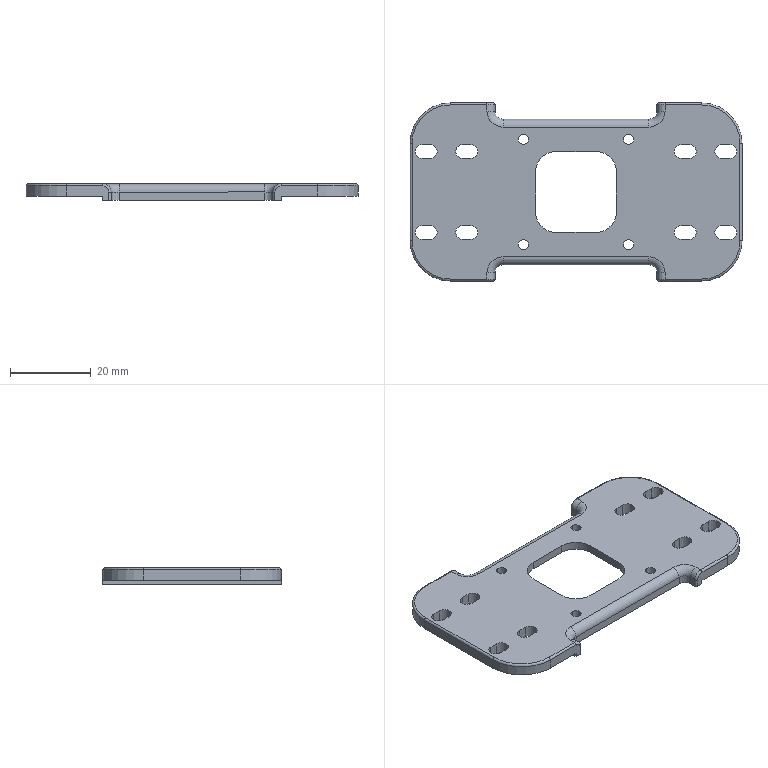NC program | NX | posted with a generic post | part box 82 x 44 x 4 mm
Whole program:
N10 G17 G21 G94 G90
(FLOOR_WALL_COPY , TOOL : D80)
N12 T19 M6
N14 G54
N16 G17 G0 G90 X-84. Y0. S5000 M3
N18 G43 Z30. H19
N20 Z3.
N22 G94 G1 Z0. F1200.
N24 X-81.
N26 X81.
N28 X84.
N30 Z3.
N32 G0 Z30.
N34 M5
(FLOOR_WALL_1 , TOOL : D4)
N36 T11 M6
N38 G54
N40 G17 G0 G90 X-44.5 Y-2.252 S9500 M3
N42 G43 Z30. H11
N44 Z0.7
N46 G94 G1 Z-0.3 F1000.
N48 X-41.2 Y-0.346
N50 G3 X-41. Y0. R0.4
N52 G1 Y12. F2500.
N54 G2 X-31. Y22. R10.
N56 G1 X-24.1
N58 Y-22.
N60 X-31.
N62 G2 X-41. Y-12. R10.
N64 G1 Y0.
N66 X-38.6
N68 Y12.001
N70 G2 X-31. Y19.6 R7.6
N72 G1 X-26.5
N74 Y-19.6
N76 X-31.
N78 G2 X-38.6 Y-12. R7.6
N80 G1 Y0.
N82 X-36.2
N84 Y12.
N86 G2 X-31. Y17.2 R5.2
N88 G1 X-28.9
N90 Y-17.2
N92 X-31.
N94 G2 X-36.2 Y-12. R5.2
N96 G1 Y0.
N98 X-33.8
N100 Y12.
N102 G2 X-31.3 Y14.784 R2.8
N104 G1 Y-14.784
N106 G2 X-33.8 Y-12. R2.8
N108 G1 Y0.
N110 G3 X-34. Y0.347 R0.4
N112 G1 Z0.7
N114 G0 X-44.5 Y-2.252 Z0.4
N116 G1 Z-0.6 F1000.
N118 X-41.2 Y-0.346
N120 G3 X-41. Y0. R0.4
N122 G1 Y12. F2500.
N124 G2 X-31. Y22. R10.
N126 G1 X-24.1
N128 Y-22.
N130 X-31.
N132 G2 X-41. Y-12. R10.
N134 G1 Y0.
N136 X-38.6
N138 Y12.001
N140 G2 X-31. Y19.6 R7.6
N142 G1 X-26.5
N144 Y-19.6
N146 X-31.
N148 G2 X-38.6 Y-12. R7.6
N150 G1 Y0.
N152 X-36.2
N154 Y12.
N156 G2 X-31. Y17.2 R5.2
N158 G1 X-28.9
N160 Y-17.2
N162 X-31.
N164 G2 X-36.2 Y-12. R5.2
N166 G1 Y0.
N168 X-33.8
N170 Y12.
N172 G2 X-31.3 Y14.784 R2.8
N174 G1 Y-14.784
N176 G2 X-33.8 Y-12. R2.8
N178 G1 Y0.
N180 G3 X-34. Y0.347 R0.4
N182 G1 Z0.4
N184 G0 X-44.5 Y-2.252 Z0.1
N186 G1 Z-0.9 F1000.
N188 X-41.2 Y-0.346
N190 G3 X-41. Y0. R0.4
N192 G1 Y12. F2500.
N194 G2 X-31. Y22. R10.
N196 G1 X-24.1
N198 Y-22.
N200 X-31.
N202 G2 X-41. Y-12. R10.
N204 G1 Y0.
N206 X-38.6
N208 Y12.001
N210 G2 X-31. Y19.6 R7.6
N212 G1 X-26.5
N214 Y-19.6
N216 X-31.
N218 G2 X-38.6 Y-12. R7.6
N220 G1 Y0.
N222 X-36.2
N224 Y12.
N226 G2 X-31. Y17.2 R5.2
N228 G1 X-28.9
N230 Y-17.2
N232 X-31.
N234 G2 X-36.2 Y-12. R5.2
N236 G1 Y0.
N238 X-33.8
N240 Y12.
N242 G2 X-31.3 Y14.784 R2.8
N244 G1 Y-14.784
N246 G2 X-33.8 Y-12. R2.8
N248 G1 Y0.
N250 G3 X-34. Y0.347 R0.4
N252 G1 Z0.1
N254 G0 Z30.
N256 X44.5 Y2.252
N258 Z0.7
N260 G1 Z-0.3 F1000.
N262 X41.2 Y0.346
N264 G3 X41. Y0. R0.4
N266 G1 Y-12. F2500.
N268 G2 X31. Y-22. R10.
N270 G1 X24.1
N272 Y22.
N274 X31.
N276 G2 X41. Y12. R10.
N278 G1 Y0.
N280 X38.6
N282 Y-12.
N284 G2 X31. Y-19.6 R7.6
N286 G1 X26.5
N288 Y19.6
N290 X31.
N292 G2 X38.6 Y12. R7.6
N294 G1 Y0.
N296 X36.2
N298 Y-12.
N300 G2 X31. Y-17.2 R5.2
N302 G1 X28.9
N304 Y17.2
N306 X31.
N308 G2 X36.2 Y12. R5.2
N310 G1 Y0.
N312 X33.8
N314 Y-12.
N316 G2 X31.3 Y-14.784 R2.8
N318 G1 Y14.784
N320 G2 X33.8 Y12. R2.8
N322 G1 Y0.
N324 G3 X34. Y-0.346 R0.4
N326 G1 Z0.7
N328 G0 X44.5 Y2.252 Z0.4
N330 G1 Z-0.6 F1000.
N332 X41.2 Y0.346
N334 G3 X41. Y0. R0.4
N336 G1 Y-12. F2500.
N338 G2 X31. Y-22. R10.
N340 G1 X24.1
N342 Y22.
N344 X31.
N346 G2 X41. Y12. R10.
N348 G1 Y0.
N350 X38.6
N352 Y-12.
N354 G2 X31. Y-19.6 R7.6
N356 G1 X26.5
N358 Y19.6
N360 X31.
N362 G2 X38.6 Y12. R7.6
N364 G1 Y0.
N366 X36.2
N368 Y-12.
N370 G2 X31. Y-17.2 R5.2
N372 G1 X28.9
N374 Y17.2
N376 X31.
N378 G2 X36.2 Y12. R5.2
N380 G1 Y0.
N382 X33.8
N384 Y-12.
N386 G2 X31.3 Y-14.784 R2.8
N388 G1 Y14.784
N390 G2 X33.8 Y12. R2.8
N392 G1 Y0.
N394 G3 X34. Y-0.346 R0.4
N396 G1 Z0.4
N398 G0 X44.5 Y2.252 Z0.1
N400 G1 Z-0.9 F1000.
N402 X41.2 Y0.346
N404 G3 X41. Y0. R0.4
N406 G1 Y-12. F2500.
N408 G2 X31. Y-22. R10.
N410 G1 X24.1
N412 Y22.
N414 X31.
N416 G2 X41. Y12. R10.
N418 G1 Y0.
N420 X38.6
N422 Y-12.
N424 G2 X31. Y-19.6 R7.6
N426 G1 X26.5
N428 Y19.6
N430 X31.
N432 G2 X38.6 Y12. R7.6
N434 G1 Y0.
N436 X36.2
N438 Y-12.
N440 G2 X31. Y-17.2 R5.2
N442 G1 X28.9
N444 Y17.2
N446 X31.
N448 G2 X36.2 Y12. R5.2
N450 G1 Y0.
N452 X33.8
N454 Y-12.
N456 G2 X31.3 Y-14.784 R2.8
N458 G1 Y14.784
N460 G2 X33.8 Y12. R2.8
N462 G1 Y0.
N464 G3 X34. Y-0.346 R0.4
N466 G1 Z0.1
N468 G0 Z30.
(FLOOR_WALL_1_COPY , TOOL : D4)
N470 X0.487 Y-0.977
N472 Z0.61
N474 G1 Z-0.39 F700.
N476 G3 X0.873 Y-0.873 R0.4
N478 G2 X1.814 Y0. R17.15 F2500.
N480 X0. Y1.814 R17.15
N482 X-1.814 Y0. R17.15
N484 X0. Y-1.814 R17.15
N486 X0.873 Y-0.873 R17.15
N488 G1 X2.57 Y-2.57
N490 G2 X6.031 Y0. R14.75
N492 X1.053 Y4.35 R14.75
N494 G1 X-1.053
N496 G2 X-6.031 Y0. R14.75
N498 X-1.053 Y-4.35 R14.75
N500 G1 X1.053
N502 G2 X2.57 Y-2.57 R14.75
N504 G1 X4.267 Y-4.267
N506 G2 X10.75 Y-0.857 R12.35
N508 G1 Y0.857
N510 G2 X2.348 Y6.75 R12.35
N512 G1 X-2.348
N514 G2 X-10.75 Y0.857 R12.35
N516 G1 Y-0.857
N518 G2 X-2.348 Y-6.75 R12.35
N520 G1 X2.348
N522 G2 X4.267 Y-4.267 R12.35
N524 G1 X5.964 Y-5.964
N526 G2 X13.15 Y-3.051 R9.95
N528 G1 Y3.051
N530 G2 X3.825 Y9.15 R9.95
N532 G1 X-3.825
N534 G2 X-13.15 Y3.051 R9.95
N536 G1 Y-3.051
N538 G2 X-3.825 Y-9.15 R9.95
N540 G1 X3.825
N542 G2 X5.964 Y-5.964 R9.95
N544 G1 X7.661 Y-7.661
N546 G2 X15.55 Y-5.894 R7.55
N548 G1 Y5.894
N550 G2 X5.591 Y11.55 R7.55
N552 G1 X-5.591
N554 G2 X-15.55 Y5.894 R7.55
N556 G1 Y-5.894
N558 G2 X-5.591 Y-11.55 R7.55
N560 G1 X5.591
N562 G2 X7.661 Y-7.661 R7.55
N564 G1 X9.358 Y-9.358
N566 G2 X17.95 Y-11.579 R5.15
N568 G1 Y11.579
N570 G2 X7.938 Y13.95 R5.15
N572 G1 X-7.938
N574 G2 X-17.95 Y11.579 R5.15
N576 G1 Y-11.579
N578 G2 X-7.938 Y-13.95 R5.15
N580 G1 X7.938
N582 G2 X9.358 Y-9.358 R5.15
N584 G3 X9.462 Y-8.972 R0.4
N586 G1 Z0.61
N588 G0 X0.487 Y-0.977 Z0.22
N590 G1 Z-0.78 F700.
N592 G3 X0.873 Y-0.873 R0.4
N594 G2 X1.814 Y0. R17.15 F2500.
N596 X0. Y1.814 R17.15
N598 X-1.814 Y0. R17.15
N600 X0. Y-1.814 R17.15
N602 X0.873 Y-0.873 R17.15
N604 G1 X2.57 Y-2.57
N606 G2 X6.031 Y0. R14.75
N608 X1.053 Y4.35 R14.75
N610 G1 X-1.053
N612 G2 X-6.031 Y0. R14.75
N614 X-1.053 Y-4.35 R14.75
N616 G1 X1.053
N618 G2 X2.57 Y-2.57 R14.75
N620 G1 X4.267 Y-4.267
N622 G2 X10.75 Y-0.857 R12.35
N624 G1 Y0.857
N626 G2 X2.348 Y6.75 R12.35
N628 G1 X-2.348
N630 G2 X-10.75 Y0.857 R12.35
N632 G1 Y-0.857
N634 G2 X-2.348 Y-6.75 R12.35
N636 G1 X2.348
N638 G2 X4.267 Y-4.267 R12.35
N640 G1 X5.964 Y-5.964
N642 G2 X13.15 Y-3.051 R9.95
N644 G1 Y3.051
N646 G2 X3.825 Y9.15 R9.95
N648 G1 X-3.825
N650 G2 X-13.15 Y3.051 R9.95
N652 G1 Y-3.051
N654 G2 X-3.825 Y-9.15 R9.95
N656 G1 X3.825
N658 G2 X5.964 Y-5.964 R9.95
N660 G1 X7.661 Y-7.661
N662 G2 X15.55 Y-5.894 R7.55
N664 G1 Y5.894
N666 G2 X5.591 Y11.55 R7.55
N668 G1 X-5.591
N670 G2 X-15.55 Y5.894 R7.55
N672 G1 Y-5.894
N674 G2 X-5.591 Y-11.55 R7.55
N676 G1 X5.591
N678 G2 X7.661 Y-7.661 R7.55
N680 G1 X9.358 Y-9.358
N682 G2 X17.95 Y-11.579 R5.15
N684 G1 Y11.579
N686 G2 X7.938 Y13.95 R5.15
N688 G1 X-7.938
N690 G2 X-17.95 Y11.579 R5.15
N692 G1 Y-11.579
N694 G2 X-7.938 Y-13.95 R5.15
N696 G1 X7.938
N698 G2 X9.358 Y-9.358 R5.15
N700 G3 X9.462 Y-8.972 R0.4
N702 G1 Z0.22
N704 G0 X0.487 Y-0.977 Z-0.17
N706 G1 Z-1.17 F700.
N708 G3 X0.873 Y-0.873 R0.4
N710 G2 X1.814 Y0. R17.15 F2500.
N712 X0. Y1.814 R17.15
N714 X-1.814 Y0. R17.15
N716 X0. Y-1.814 R17.15
N718 X0.873 Y-0.873 R17.15
N720 G1 X2.57 Y-2.57
N722 G2 X6.031 Y0. R14.75
N724 X1.053 Y4.35 R14.75
N726 G1 X-1.053
N728 G2 X-6.031 Y0. R14.75
N730 X-1.053 Y-4.35 R14.75
N732 G1 X1.053
N734 G2 X2.57 Y-2.57 R14.75
N736 G1 X4.267 Y-4.267
N738 G2 X10.75 Y-0.857 R12.35
N740 G1 Y0.857
N742 G2 X2.348 Y6.75 R12.35
N744 G1 X-2.348
N746 G2 X-10.75 Y0.857 R12.35
N748 G1 Y-0.857
N750 G2 X-2.348 Y-6.75 R12.35
N752 G1 X2.348
N754 G2 X4.267 Y-4.267 R12.35
N756 G1 X5.964 Y-5.964
N758 G2 X13.15 Y-3.051 R9.95
N760 G1 Y3.051
N762 G2 X3.825 Y9.15 R9.95
N764 G1 X-3.825
N766 G2 X-13.15 Y3.051 R9.95
N768 G1 Y-3.051
N770 G2 X-3.825 Y-9.15 R9.95
N772 G1 X3.825
N774 G2 X5.964 Y-5.964 R9.95
N776 G1 X7.661 Y-7.661
N778 G2 X15.55 Y-5.894 R7.55
N780 G1 Y5.894
N782 G2 X5.591 Y11.55 R7.55
N784 G1 X-5.591
N786 G2 X-15.55 Y5.894 R7.55
N788 G1 Y-5.894
N790 G2 X-5.591 Y-11.55 R7.55
N792 G1 X5.591
N794 G2 X7.661 Y-7.661 R7.55
N796 G1 X9.358 Y-9.358
N798 G2 X17.95 Y-11.579 R5.15
N800 G1 Y11.579
N802 G2 X7.938 Y13.95 R5.15
N804 G1 X-7.938
N806 G2 X-17.95 Y11.579 R5.15
N808 G1 Y-11.579
N810 G2 X-7.938 Y-13.95 R5.15
N812 G1 X7.938
N814 G2 X9.358 Y-9.358 R5.15
N816 G3 X9.462 Y-8.972 R0.4
N818 G1 Z-0.17
N820 G0 X0.487 Y-0.977 Z-0.56
N822 G1 Z-1.56 F700.
N824 G3 X0.873 Y-0.873 R0.4
N826 G2 X1.814 Y0. R17.15 F2500.
N828 X0. Y1.814 R17.15
N830 X-1.814 Y0. R17.15
N832 X0. Y-1.814 R17.15
N834 X0.873 Y-0.873 R17.15
N836 G1 X2.57 Y-2.57
N838 G2 X6.031 Y0. R14.75
N840 X1.053 Y4.35 R14.75
N842 G1 X-1.053
N844 G2 X-6.031 Y0. R14.75
N846 X-1.053 Y-4.35 R14.75
N848 G1 X1.053
N850 G2 X2.57 Y-2.57 R14.75
N852 G1 X4.267 Y-4.267
N854 G2 X10.75 Y-0.857 R12.35
N856 G1 Y0.857
N858 G2 X2.348 Y6.75 R12.35
N860 G1 X-2.348
N862 G2 X-10.75 Y0.857 R12.35
N864 G1 Y-0.857
N866 G2 X-2.348 Y-6.75 R12.35
N868 G1 X2.348
N870 G2 X4.267 Y-4.267 R12.35
N872 G1 X5.964 Y-5.964
N874 G2 X13.15 Y-3.051 R9.95
N876 G1 Y3.051
N878 G2 X3.825 Y9.15 R9.95
N880 G1 X-3.825
N882 G2 X-13.15 Y3.051 R9.95
N884 G1 Y-3.051
N886 G2 X-3.825 Y-9.15 R9.95
N888 G1 X3.825
N890 G2 X5.964 Y-5.964 R9.95
N892 G1 X7.661 Y-7.661
N894 G2 X15.55 Y-5.894 R7.55
N896 G1 Y5.894
N898 G2 X5.591 Y11.55 R7.55
N900 G1 X-5.591
N902 G2 X-15.55 Y5.894 R7.55
N904 G1 Y-5.894
N906 G2 X-5.591 Y-11.55 R7.55
N908 G1 X5.591
N910 G2 X7.661 Y-7.661 R7.55
N912 G1 X9.358 Y-9.358
N914 G2 X17.95 Y-11.579 R5.15
N916 G1 Y11.579
N918 G2 X7.938 Y13.95 R5.15
N920 G1 X-7.938
N922 G2 X-17.95 Y11.579 R5.15
N924 G1 Y-11.579
N926 G2 X-7.938 Y-13.95 R5.15
N928 G1 X7.938
N930 G2 X9.358 Y-9.358 R5.15
N932 G3 X9.462 Y-8.972 R0.4
N934 G1 Z-0.56
N936 G0 X0.487 Y-0.977 Z-0.95
N938 G1 Z-1.95 F700.
N940 G3 X0.873 Y-0.873 R0.4
N942 G2 X1.814 Y0. R17.15 F2500.
N944 X0. Y1.814 R17.15
N946 X-1.814 Y0. R17.15
N948 X0. Y-1.814 R17.15
N950 X0.873 Y-0.873 R17.15
N952 G1 X2.57 Y-2.57
N954 G2 X6.031 Y0. R14.75
N956 X1.053 Y4.35 R14.75
N958 G1 X-1.053
N960 G2 X-6.031 Y0. R14.75
N962 X-1.053 Y-4.35 R14.75
N964 G1 X1.053
N966 G2 X2.57 Y-2.57 R14.75
N968 G1 X4.267 Y-4.267
N970 G2 X10.75 Y-0.857 R12.35
N972 G1 Y0.857
N974 G2 X2.348 Y6.75 R12.35
N976 G1 X-2.348
N978 G2 X-10.75 Y0.857 R12.35
N980 G1 Y-0.857
N982 G2 X-2.348 Y-6.75 R12.35
N984 G1 X2.348
N986 G2 X4.267 Y-4.267 R12.35
N988 G1 X5.964 Y-5.964
N990 G2 X13.15 Y-3.051 R9.95
N992 G1 Y3.051
N994 G2 X3.825 Y9.15 R9.95
N996 G1 X-3.825
N998 G2 X-13.15 Y3.051 R9.95
N1000 G1 Y-3.051
N1002 G2 X-3.825 Y-9.15 R9.95
N1004 G1 X3.825
N1006 G2 X5.964 Y-5.964 R9.95
N1008 G1 X7.661 Y-7.661
N1010 G2 X15.55 Y-5.894 R7.55
N1012 G1 Y5.894
N1014 G2 X5.591 Y11.55 R7.55
N1016 G1 X-5.591
N1018 G2 X-15.55 Y5.894 R7.55
N1020 G1 Y-5.894
N1022 G2 X-5.591 Y-11.55 R7.55
N1024 G1 X5.591
N1026 G2 X7.661 Y-7.661 R7.55
N1028 G1 X9.358 Y-9.358
N1030 G2 X17.95 Y-11.579 R5.15
N1032 G1 Y11.579
N1034 G2 X7.938 Y13.95 R5.15
N1036 G1 X-7.938
N1038 G2 X-17.95 Y11.579 R5.15
N1040 G1 Y-11.579
N1042 G2 X-7.938 Y-13.95 R5.15
N1044 G1 X7.938
N1046 G2 X9.358 Y-9.358 R5.15
N1048 G3 X9.462 Y-8.972 R0.4
N1050 G1 Z-0.95
N1052 G0 Z30.
(FLOOR_WALL_1_COPY_COPY , TOOL : D4)
N1054 X44.5 Y1.097
N1056 Z0.
N1058 G1 Z-1. F700.
N1060 X43.2 Y0.346
N1062 G3 X43. Y0. R0.4
N1064 G1 Y-12. F1300.
N1066 G2 X31. Y-24. R12.
N1068 G1 X24.2
N1070 Y24.
N1072 X31.
N1074 G2 X43. Y12. R12.
N1076 G1 Y0.
N1078 X40.6
N1080 Y-12.
N1082 G2 X31. Y-21.6 R9.6
N1084 G1 X26.6
N1086 Y21.6
N1088 X31.
N1090 G2 X40.6 Y12. R9.6
N1092 G1 Y0.
N1094 X38.2
N1096 Y-12.
N1098 G2 X31. Y-19.2 R7.2
N1100 G1 X29.
N1102 Y19.2
N1104 X31.
N1106 G2 X38.2 Y12. R7.2
N1108 G1 Y0.
N1110 X35.8
N1112 Y-12.
N1114 G2 X31.4 Y-16.783 R4.8
N1116 G1 Y16.783
N1118 G2 X35.8 Y12. R4.8
N1120 G1 Y0.
N1122 X34.
N1124 Y-12.
N1126 G2 X33.2 Y-14.04 R3.
N1128 G1 Y14.04
N1130 G2 X34. Y12. R3.
N1132 G1 Y0.
N1134 G3 X34.2 Y-0.346 R0.4
N1136 G1 Z0.
N1138 G0 X26.198 Y25.5
N1140 G1 Z-1. F700.
N1142 X24.2 Y24.346
N1144 G3 X24. Y24. R0.4
N1146 G1 Y-24. F1300.
N1148 G3 X24.2 Y-24.346 R0.4
N1150 G1 X26.198 Y-25.5
N1152 Z0.
N1154 G0 Z30.
N1156 X9.356 Y8.866
N1158 Z-1.
N1160 G1 Z-2. F700.
N1162 G3 X9.252 Y9.252 R0.4
N1164 X17.8 Y10.753 R5.3 F1300.
N1166 G1 Y-10.753
N1168 G3 X7.761 Y-13.8 R5.3
N1170 G1 X-7.761
N1172 G3 X-17.8 Y-10.753 R5.3
N1174 G1 Y10.753
N1176 G3 X-7.761 Y13.8 R5.3
N1178 G1 X7.761
N1180 G3 X9.252 Y9.252 R5.3
N1182 G1 X7.555 Y7.555
N1184 G3 X15.4 Y5.684 R7.7
N1186 G1 Y-5.684
N1188 G3 X5.468 Y-11.4 R7.7
N1190 G1 X-5.468
N1192 G3 X-15.4 Y-5.684 R7.7
N1194 G1 Y5.684
N1196 G3 X-5.468 Y11.4 R7.7
N1198 G1 X5.468
N1200 G3 X7.555 Y7.555 R7.7
N1202 G1 X5.858 Y5.858
N1204 G3 X13. Y2.9 R10.1
N1206 G1 Y-2.9
N1208 G3 X3.726 Y-9. R10.1
N1210 G1 X-3.726
N1212 G3 X-13. Y-2.9 R10.1
N1214 G1 Y2.9
N1216 G3 X-3.726 Y9. R10.1
N1218 G1 X3.726
N1220 G3 X5.858 Y5.858 R10.1
N1222 G1 X4.161 Y4.161
N1224 G3 X10.6 Y0.733 R12.5
N1226 G1 Y-0.733
N1228 G3 X2.263 Y-6.6 R12.5
N1230 G1 X-2.263
N1232 G3 X-10.6 Y-0.733 R12.5
N1234 G1 Y0.733
N1236 G3 X-2.263 Y6.6 R12.5
N1238 G1 X2.263
N1240 G3 X4.161 Y4.161 R12.5
N1242 G1 X2.464 Y2.464
N1244 G3 X5.719 Y0. R14.9
N1246 X0.976 Y-4.2 R14.9
N1248 G1 X-0.976
N1250 G3 X-5.719 Y0. R14.9
N1252 X-0.976 Y4.2 R14.9
N1254 G1 X0.976
N1256 G3 X2.464 Y2.464 R14.9
N1258 G1 X0.767 Y0.767
N1260 G3 X1.586 Y0. R17.3
N1262 X0. Y-1.586 R17.3
N1264 X-1.586 Y0. R17.3
N1266 X0. Y1.586 R17.3
N1268 X0.767 Y0.767 R17.3
N1270 X1.153 Y0.664 R0.4
N1272 G1 Z-1.
N1274 G0 X16.3 Y-1.212
N1276 G1 Z-2. F700.
N1278 X17.8 Y-0.346
N1280 G3 X18. Y0. R0.4
N1282 G1 Y11.995 F1300.
N1284 G2 X11.995 Y8. R5.1
N1286 X7.999 Y14. R5.1
N1288 G1 X-7.999
N1290 G2 X-12. Y7.999 R5.1
N1292 X-18. Y11.995 R5.1
N1294 G1 Y-11.995
N1296 G2 X-11.995 Y-8. R5.1
N1298 X-7.999 Y-14. R5.1
N1300 G1 X7.999
N1302 G2 X12. Y-7.999 R5.1
N1304 X18. Y-11.995 R5.1
N1306 G1 Y0.
N1308 G3 X17.8 Y0.346 R0.4
N1310 G1 X16.5 Y1.097
N1312 Z-1.
N1314 G0 Z30.
N1316 X-44.5 Y-1.097
N1318 Z0.
N1320 G1 Z-1. F700.
N1322 X-43.2 Y-0.346
N1324 G3 X-43. Y0. R0.4
N1326 G1 Y12. F1300.
N1328 G2 X-31. Y24. R12.
N1330 G1 X-24.2
N1332 Y-24.
N1334 X-31.
N1336 G2 X-43. Y-12. R12.
N1338 G1 Y0.
N1340 X-40.6
N1342 Y12.
N1344 G2 X-31. Y21.6 R9.6
N1346 G1 X-26.6
N1348 Y-21.6
N1350 X-31.
N1352 G2 X-40.6 Y-12. R9.6
N1354 G1 Y0.
N1356 X-38.2
N1358 Y12.001
N1360 G2 X-31. Y19.2 R7.2
N1362 G1 X-29.
N1364 Y-19.2
N1366 X-31.
N1368 G2 X-38.2 Y-12. R7.2
N1370 G1 Y0.
N1372 X-35.8
N1374 Y12.001
N1376 G2 X-31.4 Y16.783 R4.8
N1378 G1 Y-16.783
N1380 G2 X-35.8 Y-12. R4.8
N1382 G1 Y0.
N1384 X-34.
N1386 Y12.
N1388 G2 X-33.2 Y14.04 R3.
N1390 G1 Y-14.04
N1392 G2 X-34. Y-12. R3.
N1394 G1 Y0.
N1396 G3 X-34.2 Y0.347 R0.4
N1398 G1 Z0.
N1400 G0 X-26.198 Y-25.5
N1402 G1 Z-1. F700.
N1404 X-24.2 Y-24.346
N1406 G3 X-24. Y-24. R0.4
N1408 G1 Y24. F1300.
N1410 G3 X-24.2 Y24.346 R0.4
N1412 G1 X-26.198 Y25.5
N1414 Z0.
N1416 G0 Z30.
N1418 M5
(ZLEVEL_PROFILE_COPY_1_COPY , TOOL : D3)
N1420 T16 M6
N1422 G54
N1424 G17 G0 G90 X-17.9 Y-11.092 S9500 M3
N1426 G43 Z30. H16
N1428 Z1.214
N1430 G94 G1 Z-0.286 F1000.
N1432 X-18.35 Y-11.352
N1434 G3 X-18.5 Y-11.612 R0.3
N1436 G1 Y-14. F1200.
N1438 G3 X-18. Y-14.5 R0.5
N1440 X-17.511 Y-13.902 R0.5
N1442 G2 X-17.412 Y-11.699 R4.6
N1444 G3 X-17.483 Y-11.408 R0.3
N1446 G1 X-17.821 Y-11.052
N1448 Z1.214
N1450 G0 X-17.9 Y-11.092 Z0.929
N1452 G1 Z-0.571 F1000.
N1454 X-18.35 Y-11.352
N1456 G3 X-18.5 Y-11.612 R0.3
N1458 G1 Y-14. F1200.
N1460 G3 X-18. Y-14.5 R0.5
N1462 X-17.511 Y-13.902 R0.5
N1464 G2 X-17.412 Y-11.699 R4.6
N1466 G3 X-17.483 Y-11.408 R0.3
N1468 G1 X-17.821 Y-11.052
N1470 Z0.929
N1472 G0 X-17.9 Y-11.092 Z0.643
N1474 G1 Z-0.857 F1000.
N1476 X-18.35 Y-11.352
N1478 G3 X-18.5 Y-11.612 R0.3
N1480 G1 Y-14. F1200.
N1482 G3 X-18. Y-14.5 R0.5
N1484 X-17.511 Y-13.902 R0.5
N1486 G2 X-17.412 Y-11.699 R4.6
N1488 G3 X-17.483 Y-11.408 R0.3
N1490 G1 X-17.821 Y-11.052
N1492 Z0.643
N1494 G0 X-17.9 Y-11.092 Z0.357
N1496 G1 Z-1.143 F1000.
N1498 X-18.35 Y-11.352
N1500 G3 X-18.5 Y-11.612 R0.3
N1502 G1 Y-14. F1200.
N1504 G3 X-18. Y-14.5 R0.5
N1506 X-17.511 Y-13.902 R0.5
N1508 G2 X-17.412 Y-11.699 R4.6
N1510 G3 X-17.483 Y-11.408 R0.3
N1512 G1 X-17.821 Y-11.052
N1514 Z0.357
N1516 G0 X-17.9 Y-11.092 Z0.071
N1518 G1 Z-1.429 F1000.
N1520 X-18.35 Y-11.352
N1522 G3 X-18.5 Y-11.612 R0.3
N1524 G1 Y-14. F1200.
N1526 G3 X-18. Y-14.5 R0.5
N1528 X-17.511 Y-13.902 R0.5
N1530 G2 X-17.412 Y-11.699 R4.6
N1532 G3 X-17.483 Y-11.408 R0.3
N1534 G1 X-17.821 Y-11.052
N1536 Z0.071
N1538 G0 X-17.9 Y-11.092 Z-0.214
N1540 G1 Z-1.714 F1000.
N1542 X-18.35 Y-11.352
N1544 G3 X-18.5 Y-11.612 R0.3
N1546 G1 Y-14. F1200.
N1548 G3 X-18. Y-14.5 R0.5
N1550 X-17.511 Y-13.902 R0.5
N1552 G2 X-17.412 Y-11.699 R4.6
N1554 G3 X-17.483 Y-11.408 R0.3
N1556 G1 X-17.821 Y-11.052
N1558 Z-0.214
N1560 G0 X-17.9 Y-11.092 Z-0.5
N1562 G1 Z-2. F1000.
N1564 X-18.35 Y-11.352
N1566 G3 X-18.5 Y-11.612 R0.3
N1568 G1 Y-14. F1200.
N1570 G3 X-18. Y-14.5 R0.5
N1572 X-17.511 Y-13.902 R0.5
N1574 G2 X-17.412 Y-11.699 R4.6
N1576 G3 X-17.483 Y-11.408 R0.3
N1578 G1 X-17.821 Y-11.052
N1580 Z-0.5
N1582 G0 Z30.
N1584 X17.839 Y-11.096
N1586 Z1.214
N1588 G1 Z-0.286 F1000.
N1590 X17.497 Y-11.448
N1592 G3 X17.424 Y-11.739 R0.3
N1594 G2 X17.511 Y-13.902 R4.6 F1200.
N1596 G3 X18. Y-14.5 R0.5
N1598 X18.5 Y-14. R0.5
N1600 G1 Y-11.638
N1602 G3 X18.35 Y-11.378 R0.3
N1604 G1 X17.9 Y-11.118
N1606 Z1.214
N1608 G0 X17.839 Y-11.096 Z0.929
N1610 G1 Z-0.571 F1000.
N1612 X17.497 Y-11.448
N1614 G3 X17.424 Y-11.739 R0.3
N1616 G2 X17.511 Y-13.902 R4.6 F1200.
N1618 G3 X18. Y-14.5 R0.5
N1620 X18.5 Y-14. R0.5
N1622 G1 Y-11.638
N1624 G3 X18.35 Y-11.378 R0.3
N1626 G1 X17.9 Y-11.118
N1628 Z0.929
N1630 G0 X17.839 Y-11.096 Z0.643
N1632 G1 Z-0.857 F1000.
N1634 X17.497 Y-11.448
N1636 G3 X17.424 Y-11.739 R0.3
N1638 G2 X17.511 Y-13.902 R4.6 F1200.
N1640 G3 X18. Y-14.5 R0.5
N1642 X18.5 Y-14. R0.5
N1644 G1 Y-11.638
N1646 G3 X18.35 Y-11.378 R0.3
N1648 G1 X17.9 Y-11.118
N1650 Z0.643
N1652 G0 X17.839 Y-11.096 Z0.357
N1654 G1 Z-1.143 F1000.
N1656 X17.497 Y-11.448
N1658 G3 X17.424 Y-11.739 R0.3
N1660 G2 X17.511 Y-13.902 R4.6 F1200.
N1662 G3 X18. Y-14.5 R0.5
N1664 X18.5 Y-14. R0.5
N1666 G1 Y-11.638
N1668 G3 X18.35 Y-11.378 R0.3
N1670 G1 X17.9 Y-11.118
N1672 Z0.357
N1674 G0 X17.839 Y-11.096 Z0.071
N1676 G1 Z-1.429 F1000.
N1678 X17.497 Y-11.448
N1680 G3 X17.424 Y-11.739 R0.3
N1682 G2 X17.511 Y-13.902 R4.6 F1200.
N1684 G3 X18. Y-14.5 R0.5
N1686 X18.5 Y-14. R0.5
N1688 G1 Y-11.638
N1690 G3 X18.35 Y-11.378 R0.3
N1692 G1 X17.9 Y-11.118
N1694 Z0.071
N1696 G0 X17.839 Y-11.096 Z-0.214
N1698 G1 Z-1.714 F1000.
N1700 X17.497 Y-11.448
N1702 G3 X17.424 Y-11.739 R0.3
N1704 G2 X17.511 Y-13.902 R4.6 F1200.
N1706 G3 X18. Y-14.5 R0.5
N1708 X18.5 Y-14. R0.5
N1710 G1 Y-11.638
N1712 G3 X18.35 Y-11.378 R0.3
N1714 G1 X17.9 Y-11.118
N1716 Z-0.214
N1718 G0 X17.839 Y-11.096 Z-0.5
N1720 G1 Z-2. F1000.
N1722 X17.497 Y-11.448
N1724 G3 X17.424 Y-11.739 R0.3
N1726 G2 X17.511 Y-13.902 R4.6 F1200.
N1728 G3 X18. Y-14.5 R0.5
N1730 X18.5 Y-14. R0.5
N1732 G1 Y-11.638
N1734 G3 X18.35 Y-11.378 R0.3
N1736 G1 X17.9 Y-11.118
N1738 Z-0.5
N1740 G0 Z30.
N1742 Y11.092
N1744 Z1.214
N1746 G1 Z-0.286 F1000.
N1748 X18.35 Y11.352
N1750 G3 X18.5 Y11.612 R0.3
N1752 G1 Y14. F1200.
N1754 G3 X18. Y14.5 R0.5
N1756 X17.511 Y13.902 R0.5
N1758 G2 X17.412 Y11.699 R4.6
N1760 G3 X17.483 Y11.408 R0.3
N1762 G1 X17.821 Y11.052
N1764 Z1.214
N1766 G0 X17.9 Y11.092 Z0.929
N1768 G1 Z-0.571 F1000.
N1770 X18.35 Y11.352
N1772 G3 X18.5 Y11.612 R0.3
N1774 G1 Y14. F1200.
N1776 G3 X18. Y14.5 R0.5
N1778 X17.511 Y13.902 R0.5
N1780 G2 X17.412 Y11.699 R4.6
N1782 G3 X17.483 Y11.408 R0.3
N1784 G1 X17.821 Y11.052
N1786 Z0.929
N1788 G0 X17.9 Y11.092 Z0.643
N1790 G1 Z-0.857 F1000.
N1792 X18.35 Y11.352
N1794 G3 X18.5 Y11.612 R0.3
N1796 G1 Y14. F1200.
N1798 G3 X18. Y14.5 R0.5
N1800 X17.511 Y13.902 R0.5
N1802 G2 X17.412 Y11.699 R4.6
N1804 G3 X17.483 Y11.408 R0.3
N1806 G1 X17.821 Y11.052
N1808 Z0.643
N1810 G0 X17.9 Y11.092 Z0.357
N1812 G1 Z-1.143 F1000.
N1814 X18.35 Y11.352
N1816 G3 X18.5 Y11.612 R0.3
N1818 G1 Y14. F1200.
N1820 G3 X18. Y14.5 R0.5
N1822 X17.511 Y13.902 R0.5
N1824 G2 X17.412 Y11.699 R4.6
N1826 G3 X17.483 Y11.408 R0.3
N1828 G1 X17.821 Y11.052
N1830 Z0.357
N1832 G0 X17.9 Y11.092 Z0.071
N1834 G1 Z-1.429 F1000.
N1836 X18.35 Y11.352
N1838 G3 X18.5 Y11.612 R0.3
N1840 G1 Y14. F1200.
N1842 G3 X18. Y14.5 R0.5
N1844 X17.511 Y13.902 R0.5
N1846 G2 X17.412 Y11.699 R4.6
N1848 G3 X17.483 Y11.408 R0.3
N1850 G1 X17.821 Y11.052
N1852 Z0.071
N1854 G0 X17.9 Y11.092 Z-0.214
N1856 G1 Z-1.714 F1000.
N1858 X18.35 Y11.352
N1860 G3 X18.5 Y11.612 R0.3
N1862 G1 Y14. F1200.
N1864 G3 X18. Y14.5 R0.5
N1866 X17.511 Y13.902 R0.5
N1868 G2 X17.412 Y11.699 R4.6
N1870 G3 X17.483 Y11.408 R0.3
N1872 G1 X17.821 Y11.052
N1874 Z-0.214
N1876 G0 X17.9 Y11.092 Z-0.5
N1878 G1 Z-2. F1000.
N1880 X18.35 Y11.352
N1882 G3 X18.5 Y11.612 R0.3
N1884 G1 Y14. F1200.
N1886 G3 X18. Y14.5 R0.5
N1888 X17.511 Y13.902 R0.5
N1890 G2 X17.412 Y11.699 R4.6
N1892 G3 X17.483 Y11.408 R0.3
N1894 G1 X17.821 Y11.052
N1896 Z-0.5
N1898 G0 Z30.
N1900 X-17.839 Y11.096
N1902 Z1.214
N1904 G1 Z-0.286 F1000.
N1906 X-17.497 Y11.448
N1908 G3 X-17.424 Y11.739 R0.3
N1910 G2 X-17.511 Y13.902 R4.6 F1200.
N1912 G3 X-18. Y14.5 R0.5
N1914 X-18.5 Y14. R0.5
N1916 G1 Y11.638
N1918 G3 X-18.35 Y11.378 R0.3
N1920 G1 X-17.9 Y11.118
N1922 Z1.214
N1924 G0 X-17.839 Y11.096 Z0.929
N1926 G1 Z-0.571 F1000.
N1928 X-17.497 Y11.448
N1930 G3 X-17.424 Y11.739 R0.3
N1932 G2 X-17.511 Y13.902 R4.6 F1200.
N1934 G3 X-18. Y14.5 R0.5
N1936 X-18.5 Y14. R0.5
N1938 G1 Y11.638
N1940 G3 X-18.35 Y11.378 R0.3
N1942 G1 X-17.9 Y11.118
N1944 Z0.929
N1946 G0 X-17.839 Y11.096 Z0.643
N1948 G1 Z-0.857 F1000.
N1950 X-17.497 Y11.448
N1952 G3 X-17.424 Y11.739 R0.3
N1954 G2 X-17.511 Y13.902 R4.6 F1200.
N1956 G3 X-18. Y14.5 R0.5
N1958 X-18.5 Y14. R0.5
N1960 G1 Y11.638
N1962 G3 X-18.35 Y11.378 R0.3
N1964 G1 X-17.9 Y11.118
N1966 Z0.643
N1968 G0 X-17.839 Y11.096 Z0.357
N1970 G1 Z-1.143 F1000.
N1972 X-17.497 Y11.448
N1974 G3 X-17.424 Y11.739 R0.3
N1976 G2 X-17.511 Y13.902 R4.6 F1200.
N1978 G3 X-18. Y14.5 R0.5
N1980 X-18.5 Y14. R0.5
N1982 G1 Y11.638
N1984 G3 X-18.35 Y11.378 R0.3
N1986 G1 X-17.9 Y11.118
N1988 Z0.357
N1990 G0 X-17.839 Y11.096 Z0.071
N1992 G1 Z-1.429 F1000.
N1994 X-17.497 Y11.448
N1996 G3 X-17.424 Y11.739 R0.3
N1998 G2 X-17.511 Y13.902 R4.6 F1200.
N2000 G3 X-18. Y14.5 R0.5
N2002 X-18.5 Y14. R0.5
N2004 G1 Y11.638
N2006 G3 X-18.35 Y11.378 R0.3
N2008 G1 X-17.9 Y11.118
N2010 Z0.071
N2012 G0 X-17.839 Y11.096 Z-0.214
N2014 G1 Z-1.714 F1000.
N2016 X-17.497 Y11.448
N2018 G3 X-17.424 Y11.739 R0.3
N2020 G2 X-17.511 Y13.902 R4.6 F1200.
N2022 G3 X-18. Y14.5 R0.5
N2024 X-18.5 Y14. R0.5
N2026 G1 Y11.638
N2028 G3 X-18.35 Y11.378 R0.3
N2030 G1 X-17.9 Y11.118
N2032 Z-0.214
N2034 G0 X-17.839 Y11.096 Z-0.5
N2036 G1 Z-2. F1000.
N2038 X-17.497 Y11.448
N2040 G3 X-17.424 Y11.739 R0.3
N2042 G2 X-17.511 Y13.902 R4.6 F1200.
N2044 G3 X-18. Y14.5 R0.5
N2046 X-18.5 Y14. R0.5
N2048 G1 Y11.638
N2050 G3 X-18.35 Y11.378 R0.3
N2052 G1 X-17.9 Y11.118
N2054 Z-0.5
N2056 G0 Z30.
N2058 M5
(PLANAR_MILL_2_COPY_COPY , TOOL : D6A45)
N2060 T01 M6
N2062 G54
N2064 G17 G0 G90 X-13.6 Y13.433 S9500 M3
N2066 G43 Z30. H1
N2068 Z0.5
N2070 G94 G1 Z-0.5 F1250.
N2072 G3 X-13.85 Y13. R0.5
N2074 X-13. Y12.15 R0.85
N2076 X-13.85 Y13. R-0.85
N2078 X-13.6 Y12.567 R0.5
N2080 G1 Z0.5
N2082 G0 Z30.
N2084 X-19.1 Y0.866
N2086 Z0.5
N2088 G1 Z-0.5
N2090 G3 X-19.6 Y0. R1.
N2092 G1 Y-14.
N2094 G3 X-18. Y-15.6 R1.6
N2096 X-16.432 Y-13.686 R1.6
N2098 G2 X-9.568 Y-13.686 R-3.5
N2100 G3 X-7.999 Y-15.6 R1.6
N2102 G1 X7.999
N2104 G3 X9.568 Y-13.686 R1.6
N2106 G2 X16.432 Y-13.686 R-3.5
N2108 G3 X18. Y-15.6 R1.6
N2110 X19.6 Y-14. R1.6
N2112 G1 Y14.
N2114 G3 X18. Y15.6 R1.6
N2116 X16.432 Y13.686 R1.6
N2118 G2 X9.568 Y13.686 R-3.5
N2120 G3 X7.999 Y15.6 R1.6
N2122 G1 X-7.999
N2124 G3 X-9.568 Y13.686 R1.6
N2126 G2 X-16.432 Y13.686 R-3.5
N2128 G3 X-18. Y15.6 R1.6
N2130 X-19.6 Y14. R1.6
N2132 G1 Y0.
N2134 G3 X-19.1 Y-0.866 R1.
N2136 G1 Z0.5
N2138 G0 Z30.
N2140 X13.6 Y12.567
N2142 Z0.5
N2144 G1 Z-0.5
N2146 G3 X13.85 Y13. R0.5
N2148 X13. Y13.85 R0.85
N2150 X13.85 Y13. R-0.85
N2152 X13.6 Y13.433 R0.5
N2154 G1 Z0.5
N2156 G0 Z30.
N2158 X22.9 Y0.866
N2160 Z0.5
N2162 G1 Z-0.5
N2164 G3 X22.4 Y0. R1.
N2166 G1 Y-22.
N2168 G2 X22. Y-22.4 R0.4
N2170 G1 X20.5
N2172 G2 X19.6 Y-21.5 R0.9
N2174 G1 Y-20.
N2176 G3 X18. Y-18.4 R1.6
N2178 G1 X-18.
N2180 G3 X-19.6 Y-20. R1.6
N2182 G1 Y-21.5
N2184 G2 X-20.5 Y-22.4 R0.9
N2186 G1 X-22.
N2188 G2 X-22.4 Y-22. R0.4
N2190 G1 Y22.
N2192 G2 X-22. Y22.4 R0.4
N2194 G1 X-20.5
N2196 G2 X-19.6 Y21.5 R0.9
N2198 G1 Y20.
N2200 G3 X-18. Y18.4 R1.6
N2202 G1 X18.
N2204 G3 X19.6 Y20. R1.6
N2206 G1 Y21.5
N2208 G2 X20.5 Y22.4 R0.9
N2210 G1 X22.
N2212 G2 X22.4 Y22. R0.4
N2214 G1 Y0.
N2216 G3 X22.9 Y-0.866 R1.
N2218 G1 Z0.5
N2220 G0 Z30.
N2222 X13.6 Y-13.433
N2224 Z0.5
N2226 G1 Z-0.5
N2228 G3 X13.85 Y-13. R0.5
N2230 X13. Y-12.15 R0.85
N2232 X13.85 Y-13. R-0.85
N2234 X13.6 Y-12.567 R0.5
N2236 G1 Z0.5
N2238 G0 Z30.
N2240 X-13.6
N2242 Z0.5
N2244 G1 Z-0.5
N2246 G3 X-13.85 Y-13. R0.5
N2248 X-13. Y-13.85 R0.85
N2250 X-13.85 Y-13. R-0.85
N2252 X-13.6 Y-13.433 R0.5
N2254 G1 Z0.5
N2256 G0 Z30.
(PLANAR_MILL_2_COPY_COPY_COPY , TOOL : D6A45)
N2258 X-9.1 Y0.866
N2260 Z-1.5
N2262 G1 Z-2.5
N2264 G3 X-9.6 Y0. R1.
N2266 G1 Y-5.
N2268 G3 X-5. Y-9.6 R4.6
N2270 G1 X5.
N2272 G3 X9.6 Y-5. R4.6
N2274 G1 Y5.
N2276 G3 X5. Y9.6 R4.6
N2278 G1 X-5.
N2280 G3 X-9.6 Y5. R4.6
N2282 G1 Y0.
N2284 G3 X-9.1 Y-0.866 R1.
N2286 G1 Z-1.5
N2288 G0 Z30.
(PLANAR_MILL_2_COPY_COPY_COPY_COPY , TOOL : D6A45)
N2290 X-26.699 Y10.3
N2292 Z0.
N2294 G1 X-28.137 Z-0.386
N2296 X-28.3 Y10.137 Z-0.447
N2298 Y9.863 Z-0.521
N2300 X-28.137 Y9.7 Z-0.582
N2302 X-25.863 Z-1.192
N2304 X-25.7 Y9.863 Z-1.254
N2306 Y10.137 Z-1.327
N2308 X-25.863 Y10.3 Z-1.389
N2310 X-28.137 Z-1.998
N2312 X-28.3 Y10.137 Z-2.06
N2314 Y9.863 Z-2.134
N2316 X-28.137 Y9.7 Z-2.195
N2318 X-27. Z-2.5
N2320 X-26.
N2322 G3 X-25.7 Y10. R0.3
N2324 X-26. Y10.3 R0.3
N2326 G1 X-28.
N2328 G3 X-28.3 Y10. R0.3
N2330 X-28. Y9.7 R0.3
N2332 G1 X-27.
N2334 G3 X-26.134 Y10.2 R1.
N2336 G1 Z-1.5
N2338 G0 Z30.
N2340 X-36.699 Y10.3
N2342 Z0.
N2344 G1 X-38.137 Z-0.386
N2346 X-38.3 Y10.137 Z-0.447
N2348 Y9.863 Z-0.521
N2350 X-38.137 Y9.7 Z-0.582
N2352 X-35.863 Z-1.192
N2354 X-35.7 Y9.863 Z-1.254
N2356 Y10.137 Z-1.327
N2358 X-35.863 Y10.3 Z-1.389
N2360 X-38.137 Z-1.998
N2362 X-38.3 Y10.137 Z-2.06
N2364 Y9.863 Z-2.134
N2366 X-38.137 Y9.7 Z-2.195
N2368 X-37. Z-2.5
N2370 X-36.
N2372 G3 X-35.7 Y10. R0.3
N2374 X-36. Y10.3 R0.3
N2376 G1 X-38.
N2378 G3 X-38.3 Y10. R0.3
N2380 X-38. Y9.7 R0.3
N2382 G1 X-37.
N2384 G3 X-36.134 Y10.2 R1.
N2386 G1 Z-1.5
N2388 G0 Z30.
N2390 X-37.301 Y-10.3
N2392 Z0.
N2394 G1 X-35.863 Z-0.386
N2396 X-35.7 Y-10.137 Z-0.447
N2398 Y-9.863 Z-0.521
N2400 X-35.863 Y-9.7 Z-0.582
N2402 X-38.137 Z-1.192
N2404 X-38.3 Y-9.863 Z-1.254
N2406 Y-10.137 Z-1.327
N2408 X-38.137 Y-10.3 Z-1.389
N2410 X-35.863 Z-1.998
N2412 X-35.7 Y-10.137 Z-2.06
N2414 Y-9.863 Z-2.134
N2416 X-35.863 Y-9.7 Z-2.195
N2418 X-37. Z-2.5
N2420 X-38.
N2422 G3 X-38.3 Y-10. R0.3
N2424 X-38. Y-10.3 R0.3
N2426 G1 X-36.
N2428 G3 X-35.7 Y-10. R0.3
N2430 X-36. Y-9.7 R0.3
N2432 G1 X-37.
N2434 G3 X-37.866 Y-10.2 R1.
N2436 G1 Z-1.5
N2438 G0 Z30.
N2440 X-26.699 Y-9.7
N2442 Z0.
N2444 G1 X-28.137 Z-0.386
N2446 X-28.3 Y-9.863 Z-0.447
N2448 Y-10.137 Z-0.521
N2450 X-28.137 Y-10.3 Z-0.582
N2452 X-25.863 Z-1.192
N2454 X-25.7 Y-10.137 Z-1.254
N2456 Y-9.863 Z-1.327
N2458 X-25.863 Y-9.7 Z-1.389
N2460 X-28.137 Z-1.998
N2462 X-28.3 Y-9.863 Z-2.06
N2464 Y-10.137 Z-2.134
N2466 X-28.137 Y-10.3 Z-2.195
N2468 X-27. Z-2.5
N2470 X-26.
N2472 G3 X-25.7 Y-10. R0.3
N2474 X-26. Y-9.7 R0.3
N2476 G1 X-28.
N2478 G3 X-28.3 Y-10. R0.3
N2480 X-28. Y-10.3 R0.3
N2482 G1 X-27.
N2484 G3 X-26.134 Y-9.8 R1.
N2486 G1 Z-1.5
N2488 G0 Z30.
N2490 X-25.019 Y-24.92
N2492 Z-1.5
N2494 G1 Z-2.5
N2496 X-24.691 Y-24.399
N2498 G3 X-24.653 Y-23.4 R1.
N2500 G1 X-31.
N2502 G2 X-42.4 Y-12. R11.4
N2504 G1 Y12.
N2506 G2 X-31. Y23.4 R11.4
N2508 G1 X-24.653
N2510 G3 X-24.691 Y24.399 R1.
N2512 G1 X-25.019 Y24.92
N2514 Z-1.5
N2516 G0 Z30.
N2518 X25.019
N2520 Z-1.5
N2522 G1 Z-2.5
N2524 X24.691 Y24.399
N2526 G3 X24.653 Y23.4 R1.
N2528 G1 X31.
N2530 G2 X42.4 Y12. R11.4
N2532 G1 Y-12.
N2534 G2 X31. Y-23.4 R11.4
N2536 G1 X24.653
N2538 G3 X24.691 Y-24.399 R1.
N2540 G1 X25.019 Y-24.92
N2542 Z-1.5
N2544 G0 Z30.
N2546 X27.301 Y-9.7
N2548 Z0.
N2550 G1 X25.863 Z-0.386
N2552 X25.7 Y-9.863 Z-0.447
N2554 Y-10.137 Z-0.521
N2556 X25.863 Y-10.3 Z-0.582
N2558 X28.137 Z-1.192
N2560 X28.3 Y-10.137 Z-1.254
N2562 Y-9.863 Z-1.327
N2564 X28.137 Y-9.7 Z-1.389
N2566 X25.863 Z-1.998
N2568 X25.7 Y-9.863 Z-2.06
N2570 Y-10.137 Z-2.134
N2572 X25.863 Y-10.3 Z-2.195
N2574 X27. Z-2.5
N2576 X28.
N2578 G3 X28.3 Y-10. R0.3
N2580 X28. Y-9.7 R0.3
N2582 G1 X26.
N2584 G3 X25.7 Y-10. R0.3
N2586 X26. Y-10.3 R0.3
N2588 G1 X27.
N2590 G3 X27.866 Y-9.8 R1.
N2592 G1 Z-1.5
N2594 G0 Z30.
N2596 X36.699 Y-10.3
N2598 Z0.
N2600 G1 X38.137 Z-0.386
N2602 X38.3 Y-10.137 Z-0.447
N2604 Y-9.863 Z-0.521
N2606 X38.137 Y-9.7 Z-0.582
N2608 X35.863 Z-1.192
N2610 X35.7 Y-9.863 Z-1.254
N2612 Y-10.137 Z-1.327
N2614 X35.863 Y-10.3 Z-1.389
N2616 X38.137 Z-1.998
N2618 X38.3 Y-10.137 Z-2.06
N2620 Y-9.863 Z-2.134
N2622 X38.137 Y-9.7 Z-2.195
N2624 X37. Z-2.5
N2626 X36.
N2628 G3 X35.7 Y-10. R0.3
N2630 X36. Y-10.3 R0.3
N2632 G1 X38.
N2634 G3 X38.3 Y-10. R0.3
N2636 X38. Y-9.7 R0.3
N2638 G1 X37.
N2640 G3 X36.134 Y-10.2 R1.
N2642 G1 Z-1.5
N2644 G0 Z30.
N2646 X37.301 Y10.3
N2648 Z0.
N2650 G1 X35.863 Z-0.386
N2652 X35.7 Y10.137 Z-0.447
N2654 Y9.863 Z-0.521
N2656 X35.863 Y9.7 Z-0.582
N2658 X38.137 Z-1.192
N2660 X38.3 Y9.863 Z-1.254
N2662 Y10.137 Z-1.327
N2664 X38.137 Y10.3 Z-1.389
N2666 X35.863 Z-1.998
N2668 X35.7 Y10.137 Z-2.06
N2670 Y9.863 Z-2.134
N2672 X35.863 Y9.7 Z-2.195
N2674 X37. Z-2.5
N2676 X38.
N2678 G3 X38.3 Y10. R0.3
N2680 X38. Y10.3 R0.3
N2682 G1 X36.
N2684 G3 X35.7 Y10. R0.3
N2686 X36. Y9.7 R0.3
N2688 G1 X37.
N2690 G3 X37.866 Y10.2 R1.
N2692 G1 Z-1.5
N2694 G0 Z30.
N2696 X26.699 Y9.7
N2698 Z0.
N2700 G1 X28.137 Z-0.386
N2702 X28.3 Y9.863 Z-0.447
N2704 Y10.137 Z-0.521
N2706 X28.137 Y10.3 Z-0.582
N2708 X25.863 Z-1.192
N2710 X25.7 Y10.137 Z-1.254
N2712 Y9.863 Z-1.327
N2714 X25.863 Y9.7 Z-1.389
N2716 X28.137 Z-1.998
N2718 X28.3 Y9.863 Z-2.06
N2720 Y10.137 Z-2.134
N2722 X28.137 Y10.3 Z-2.195
N2724 X27. Z-2.5
N2726 X26.
N2728 G3 X25.7 Y10. R0.3
N2730 X26. Y9.7 R0.3
N2732 G1 X28.
N2734 G3 X28.3 Y10. R0.3
N2736 X28. Y10.3 R0.3
N2738 G1 X27.
N2740 G3 X26.134 Y9.8 R1.
N2742 G1 Z-1.5
N2744 G0 Z30.
N2746 M5
N2748 M2